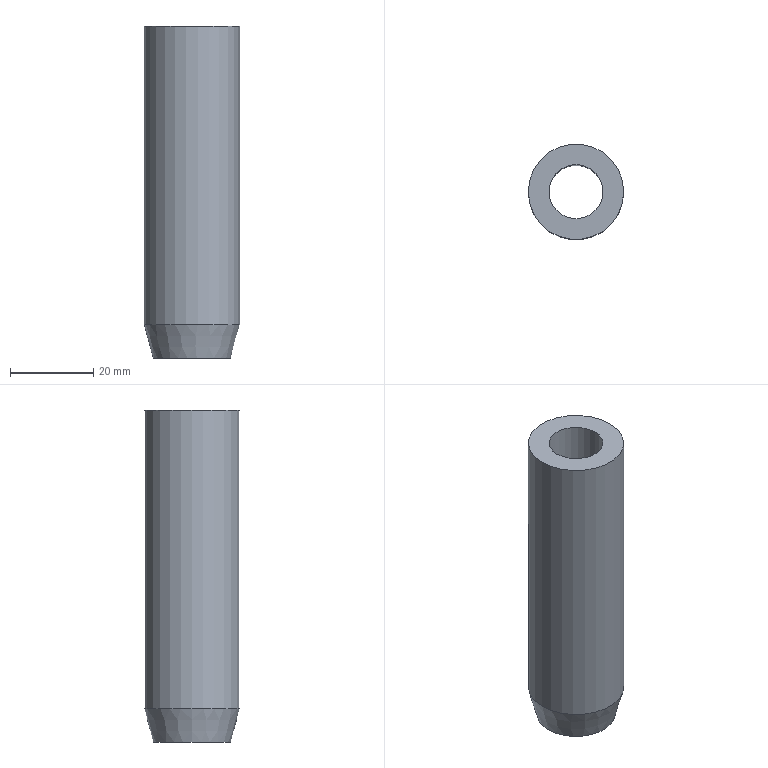Part | NX | features solid 2 | 1 solid | 5 faces | box 23 x 23 x 80 mm | volume 22038 mm3 | plane 2 | cylinder 2 | cone 1 | commonest cylinder face diameters 13 x1 23 x1
STEP:
#1=CARTESIAN_POINT('',(-244.636,655.,240.));
#2=VERTEX_POINT('',#1);
#3=CARTESIAN_POINT('',(-235.279,655.,240.));
#4=DIRECTION('',(0.,0.,-1.));
#5=DIRECTION('',(-1.,0.,0.));
#6=AXIS2_PLACEMENT_3D('',#3,#4,#5);
#7=CIRCLE('',#6,9.356);
#8=EDGE_CURVE('',#2,#2,#7,.F.);
#9=ORIENTED_EDGE('',*,*,#8,.F.);
#10=EDGE_LOOP('',(#9));
#11=FACE_BOUND('',#10,.T.);
#12=CARTESIAN_POINT('',(-241.779,655.,240.));
#13=VERTEX_POINT('',#12);
#14=CARTESIAN_POINT('',(-235.279,655.,240.));
#15=DIRECTION('',(0.,0.,-1.));
#16=DIRECTION('',(-1.,0.,0.));
#17=AXIS2_PLACEMENT_3D('',#14,#15,#16);
#18=CIRCLE('',#17,6.5);
#19=EDGE_CURVE('',#13,#13,#18,.T.);
#20=ORIENTED_EDGE('',*,*,#19,.F.);
#21=EDGE_LOOP('',(#20));
#22=FACE_BOUND('',#21,.T.);
#23=CARTESIAN_POINT('',(-235.279,655.,240.));
#24=DIRECTION('',(0.,0.,1.));
#25=DIRECTION('',(-1.,0.,0.));
#26=AXIS2_PLACEMENT_3D('',#23,#24,#25);
#27=PLANE('',#26);
#28=ADVANCED_FACE('',(#11,#22),#27,.F.);
#29=CARTESIAN_POINT('',(-223.779,655.,320.));
#30=VERTEX_POINT('',#29);
#31=CARTESIAN_POINT('',(-235.279,655.,320.));
#32=DIRECTION('',(0.,0.,-1.));
#33=DIRECTION('',(1.,0.,0.));
#34=AXIS2_PLACEMENT_3D('',#31,#32,#33);
#35=CIRCLE('',#34,11.5);
#36=EDGE_CURVE('',#30,#30,#35,.T.);
#37=ORIENTED_EDGE('',*,*,#36,.T.);
#38=EDGE_LOOP('',(#37));
#39=FACE_BOUND('',#38,.T.);
#40=CARTESIAN_POINT('',(-246.779,655.,248.));
#41=VERTEX_POINT('',#40);
#42=CARTESIAN_POINT('',(-235.279,655.,248.));
#43=DIRECTION('',(0.,0.,-1.));
#44=DIRECTION('',(-1.,0.,0.));
#45=AXIS2_PLACEMENT_3D('',#42,#43,#44);
#46=CIRCLE('',#45,11.5);
#47=EDGE_CURVE('',#41,#41,#46,.T.);
#48=ORIENTED_EDGE('',*,*,#47,.F.);
#49=EDGE_LOOP('',(#48));
#50=FACE_BOUND('',#49,.T.);
#51=CARTESIAN_POINT('',(-235.279,655.,340.));
#52=DIRECTION('',(0.,0.,-1.));
#53=DIRECTION('',(1.,0.,0.));
#54=AXIS2_PLACEMENT_3D('',#51,#52,#53);
#55=CYLINDRICAL_SURFACE('',#54,11.5);
#56=ADVANCED_FACE('',(#39,#50),#55,.T.);
#57=CARTESIAN_POINT('',(-228.779,655.,320.));
#58=VERTEX_POINT('',#57);
#59=CARTESIAN_POINT('',(-235.279,655.,320.));
#60=DIRECTION('',(0.,0.,-1.));
#61=DIRECTION('',(1.,0.,0.));
#62=AXIS2_PLACEMENT_3D('',#59,#60,#61);
#63=CIRCLE('',#62,6.5);
#64=EDGE_CURVE('',#58,#58,#63,.T.);
#65=ORIENTED_EDGE('',*,*,#64,.F.);
#66=EDGE_LOOP('',(#65));
#67=FACE_BOUND('',#66,.T.);
#68=ORIENTED_EDGE('',*,*,#19,.T.);
#69=EDGE_LOOP('',(#68));
#70=FACE_BOUND('',#69,.T.);
#71=CARTESIAN_POINT('',(-235.279,655.,340.));
#72=DIRECTION('',(0.,0.,-1.));
#73=DIRECTION('',(1.,0.,0.));
#74=AXIS2_PLACEMENT_3D('',#71,#72,#73);
#75=CYLINDRICAL_SURFACE('',#74,6.5);
#76=ADVANCED_FACE('',(#67,#70),#75,.F.);
#77=ORIENTED_EDGE('',*,*,#8,.T.);
#78=EDGE_LOOP('',(#77));
#79=FACE_BOUND('',#78,.T.);
#80=ORIENTED_EDGE('',*,*,#47,.T.);
#81=EDGE_LOOP('',(#80));
#82=FACE_BOUND('',#81,.T.);
#83=CARTESIAN_POINT('',(-235.279,655.,248.));
#84=DIRECTION('',(0.,0.,1.));
#85=DIRECTION('',(-1.,0.,0.));
#86=AXIS2_PLACEMENT_3D('',#83,#84,#85);
#87=CONICAL_SURFACE('',#86,11.5,0.2618);
#88=ADVANCED_FACE('',(#79,#82),#87,.T.);
#89=ORIENTED_EDGE('',*,*,#64,.T.);
#90=EDGE_LOOP('',(#89));
#91=FACE_BOUND('',#90,.T.);
#92=ORIENTED_EDGE('',*,*,#36,.F.);
#93=EDGE_LOOP('',(#92));
#94=FACE_BOUND('',#93,.T.);
#95=CARTESIAN_POINT('',(-755.279,85.,320.));
#96=DIRECTION('',(0.,0.,-1.));
#97=DIRECTION('',(1.,0.,0.));
#98=AXIS2_PLACEMENT_3D('',#95,#96,#97);
#99=PLANE('',#98);
#100=ADVANCED_FACE('',(#91,#94),#99,.F.);
#101=CLOSED_SHELL('',(#28,#56,#76,#88,#100));
#102=MANIFOLD_SOLID_BREP('',#101);
#103=(LENGTH_UNIT()NAMED_UNIT(*)SI_UNIT(.MILLI.,.METRE.));
#104=UNCERTAINTY_MEASURE_WITH_UNIT(LENGTH_MEASURE(0.00001),#103,'','');
#105=(NAMED_UNIT(*)PLANE_ANGLE_UNIT()SI_UNIT($,.RADIAN.));
#106=(NAMED_UNIT(*)SI_UNIT($,.STERADIAN.)SOLID_ANGLE_UNIT());
#107=(GEOMETRIC_REPRESENTATION_CONTEXT(3)GLOBAL_UNCERTAINTY_ASSIGNED_CONTEXT((#104))GLOBAL_UNIT_ASSIGNED_CONTEXT((#103,#105,#106))REPRESENTATION_CONTEXT('',''));
#108=ADVANCED_BREP_SHAPE_REPRESENTATION('',(#102),#107);